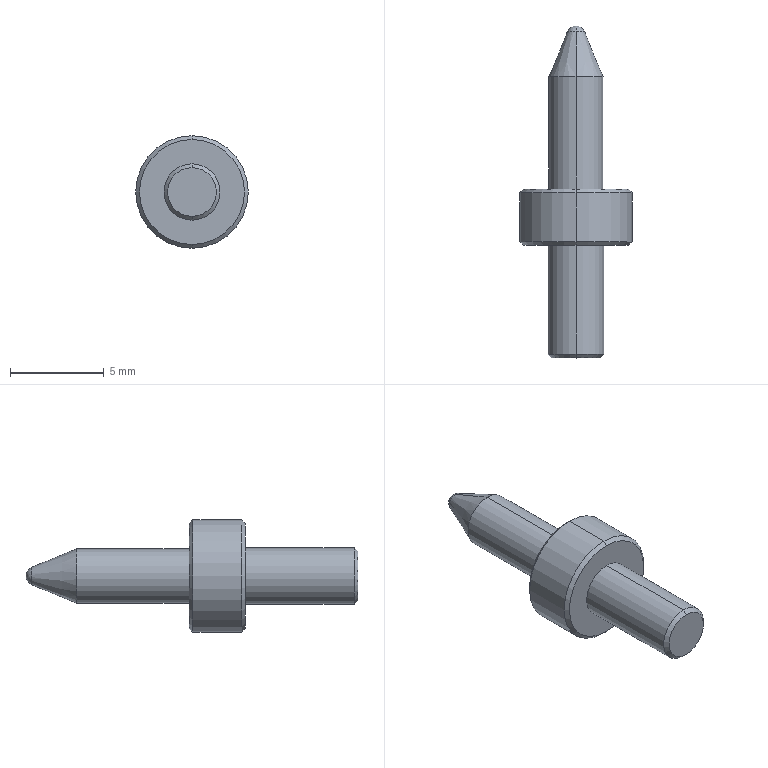Part | STEP file | PN_0028 Pin_Default | 1 solid | 19 faces | box 6 x 17.694 x 6 mm | volume 173.525 mm3 | cone 8 | cylinder 6 | plane 3 | sphere 2 | commonest cylinder face diameters 2.9 x2 3 x2 6 x2
STEP:
#1=CARTESIAN_POINT('',(0.,0.,0.));
#2=DIRECTION('',(0.,0.,1.));
#3=DIRECTION('',(1.,0.,0.));
#4=AXIS2_PLACEMENT_3D('',#1,#2,#3);
#5=CARTESIAN_POINT('',(0.,-6.,-1.3));
#6=VERTEX_POINT('',#5);
#7=CARTESIAN_POINT('',(0.,-6.,1.3));
#8=VERTEX_POINT('',#7);
#9=CARTESIAN_POINT('',(0.,-6.,0.));
#10=DIRECTION('',(0.,-1.,0.));
#11=DIRECTION('',(0.,0.,-1.));
#12=AXIS2_PLACEMENT_3D('',#9,#10,#11);
#13=CIRCLE('',#12,1.3);
#14=CARTESIAN_POINT('',(0.,-6.,0.));
#15=DIRECTION('',(0.,1.,0.));
#16=DIRECTION('',(0.,0.,1.));
#17=AXIS2_PLACEMENT_3D('',#14,#15,#16);
#18=CONICAL_SURFACE('',#17,1.3,0.7854);
#19=CARTESIAN_POINT('',(3.142,0.));
#20=DIRECTION('',(-1.,0.));
#21=VECTOR('',#20,1.);
#22=LINE('',#19,#21);
#23=(GEOMETRIC_REPRESENTATION_CONTEXT(2)PARAMETRIC_REPRESENTATION_CONTEXT()REPRESENTATION_CONTEXT('',''));
#24=DEFINITIONAL_REPRESENTATION('',(#22),#23);
#25=PCURVE('',#18,#24);
#26=CARTESIAN_POINT('',(0.,-6.,0.));
#27=DIRECTION('',(0.,-1.,0.));
#28=DIRECTION('',(0.,0.,-1.));
#29=AXIS2_PLACEMENT_3D('',#26,#27,#28);
#30=PLANE('',#29);
#31=CARTESIAN_POINT('',(0.,0.));
#32=DIRECTION('',(1.,0.));
#33=AXIS2_PLACEMENT_2D('',#31,#32);
#34=CIRCLE('',#33,1.3);
#35=(GEOMETRIC_REPRESENTATION_CONTEXT(2)PARAMETRIC_REPRESENTATION_CONTEXT()REPRESENTATION_CONTEXT('',''));
#36=DEFINITIONAL_REPRESENTATION('',(#34),#35);
#37=PCURVE('',#30,#36);
#38=SURFACE_CURVE('',#13,(#25,#37),.PCURVE_S1.);
#39=EDGE_CURVE('',#6,#8,#38,.T.);
#40=ORIENTED_EDGE('',*,*,#39,.F.);
#41=CARTESIAN_POINT('',(0.,-5.8,-1.5));
#42=VERTEX_POINT('',#41);
#43=CARTESIAN_POINT('',(0.,-6.,-1.3));
#44=DIRECTION('',(0.,0.7071,-0.7071));
#45=VECTOR('',#44,1.);
#46=LINE('',#43,#45);
#47=CARTESIAN_POINT('',(3.142,0.));
#48=DIRECTION('',(0.,1.));
#49=VECTOR('',#48,1.);
#50=LINE('',#47,#49);
#51=(GEOMETRIC_REPRESENTATION_CONTEXT(2)PARAMETRIC_REPRESENTATION_CONTEXT()REPRESENTATION_CONTEXT('',''));
#52=DEFINITIONAL_REPRESENTATION('',(#50),#51);
#53=PCURVE('',#18,#52);
#54=CARTESIAN_POINT('',(0.,-6.,0.));
#55=DIRECTION('',(0.,1.,0.));
#56=DIRECTION('',(0.,0.,1.));
#57=AXIS2_PLACEMENT_3D('',#54,#55,#56);
#58=CONICAL_SURFACE('',#57,1.3,0.7854);
#59=CARTESIAN_POINT('',(3.142,0.));
#60=DIRECTION('',(0.,1.));
#61=VECTOR('',#60,1.);
#62=LINE('',#59,#61);
#63=(GEOMETRIC_REPRESENTATION_CONTEXT(2)PARAMETRIC_REPRESENTATION_CONTEXT()REPRESENTATION_CONTEXT('',''));
#64=DEFINITIONAL_REPRESENTATION('',(#62),#63);
#65=PCURVE('',#58,#64);
#66=SURFACE_CURVE('',#46,(#53,#65),.PCURVE_S1.);
#67=EDGE_CURVE('',#6,#42,#66,.T.);
#68=ORIENTED_EDGE('',*,*,#67,.T.);
#69=CARTESIAN_POINT('',(0.,-5.8,1.5));
#70=VERTEX_POINT('',#69);
#71=CARTESIAN_POINT('',(0.,-5.8,0.));
#72=DIRECTION('',(0.,1.,0.));
#73=DIRECTION('',(0.,0.,-1.));
#74=AXIS2_PLACEMENT_3D('',#71,#72,#73);
#75=CIRCLE('',#74,1.5);
#76=CARTESIAN_POINT('',(-3.142,0.2));
#77=DIRECTION('',(1.,0.));
#78=VECTOR('',#77,1.);
#79=LINE('',#76,#78);
#80=(GEOMETRIC_REPRESENTATION_CONTEXT(2)PARAMETRIC_REPRESENTATION_CONTEXT()REPRESENTATION_CONTEXT('',''));
#81=DEFINITIONAL_REPRESENTATION('',(#79),#80);
#82=PCURVE('',#18,#81);
#83=CARTESIAN_POINT('',(0.,-6.,0.));
#84=DIRECTION('',(0.,1.,0.));
#85=DIRECTION('',(0.,0.,1.));
#86=AXIS2_PLACEMENT_3D('',#83,#84,#85);
#87=CYLINDRICAL_SURFACE('',#86,1.5);
#88=CARTESIAN_POINT('',(-3.142,0.2));
#89=DIRECTION('',(1.,0.));
#90=VECTOR('',#89,1.);
#91=LINE('',#88,#90);
#92=(GEOMETRIC_REPRESENTATION_CONTEXT(2)PARAMETRIC_REPRESENTATION_CONTEXT()REPRESENTATION_CONTEXT('',''));
#93=DEFINITIONAL_REPRESENTATION('',(#91),#92);
#94=PCURVE('',#87,#93);
#95=SURFACE_CURVE('',#75,(#82,#94),.PCURVE_S1.);
#96=EDGE_CURVE('',#70,#42,#95,.T.);
#97=ORIENTED_EDGE('',*,*,#96,.F.);
#98=CARTESIAN_POINT('',(0.,-6.,1.3));
#99=DIRECTION('',(0.,0.7071,0.7071));
#100=VECTOR('',#99,1.);
#101=LINE('',#98,#100);
#102=CARTESIAN_POINT('',(0.,0.));
#103=DIRECTION('',(0.,1.));
#104=VECTOR('',#103,1.);
#105=LINE('',#102,#104);
#106=(GEOMETRIC_REPRESENTATION_CONTEXT(2)PARAMETRIC_REPRESENTATION_CONTEXT()REPRESENTATION_CONTEXT('',''));
#107=DEFINITIONAL_REPRESENTATION('',(#105),#106);
#108=PCURVE('',#18,#107);
#109=CARTESIAN_POINT('',(6.283,0.));
#110=DIRECTION('',(0.,1.));
#111=VECTOR('',#110,1.);
#112=LINE('',#109,#111);
#113=(GEOMETRIC_REPRESENTATION_CONTEXT(2)PARAMETRIC_REPRESENTATION_CONTEXT()REPRESENTATION_CONTEXT('',''));
#114=DEFINITIONAL_REPRESENTATION('',(#112),#113);
#115=PCURVE('',#58,#114);
#116=SURFACE_CURVE('',#101,(#108,#115),.PCURVE_S1.);
#117=EDGE_CURVE('',#8,#70,#116,.T.);
#118=ORIENTED_EDGE('',*,*,#117,.F.);
#119=EDGE_LOOP('',(#40,#68,#97,#118));
#120=FACE_BOUND('',#119,.T.);
#121=ADVANCED_FACE('',(#120),#18,.T.);
#122=CARTESIAN_POINT('',(0.,0.,-2.8));
#123=VERTEX_POINT('',#122);
#124=CARTESIAN_POINT('',(0.,0.,2.8));
#125=VERTEX_POINT('',#124);
#126=CARTESIAN_POINT('',(0.,0.,0.));
#127=DIRECTION('',(0.,-1.,0.));
#128=DIRECTION('',(0.,0.,-1.));
#129=AXIS2_PLACEMENT_3D('',#126,#127,#128);
#130=CIRCLE('',#129,2.8);
#131=CARTESIAN_POINT('',(0.,0.2,0.));
#132=DIRECTION('',(0.,1.,0.));
#133=DIRECTION('',(0.,0.,1.));
#134=AXIS2_PLACEMENT_3D('',#131,#132,#133);
#135=CONICAL_SURFACE('',#134,3.,0.7854);
#136=CARTESIAN_POINT('',(3.142,-0.2));
#137=DIRECTION('',(-1.,0.));
#138=VECTOR('',#137,1.);
#139=LINE('',#136,#138);
#140=(GEOMETRIC_REPRESENTATION_CONTEXT(2)PARAMETRIC_REPRESENTATION_CONTEXT()REPRESENTATION_CONTEXT('',''));
#141=DEFINITIONAL_REPRESENTATION('',(#139),#140);
#142=PCURVE('',#135,#141);
#143=CARTESIAN_POINT('',(0.,0.,3.));
#144=DIRECTION('',(0.,-1.,0.));
#145=DIRECTION('',(0.,0.,-1.));
#146=AXIS2_PLACEMENT_3D('',#143,#144,#145);
#147=PLANE('',#146);
#148=CARTESIAN_POINT('',(3.,0.));
#149=DIRECTION('',(1.,0.));
#150=AXIS2_PLACEMENT_2D('',#148,#149);
#151=CIRCLE('',#150,2.8);
#152=(GEOMETRIC_REPRESENTATION_CONTEXT(2)PARAMETRIC_REPRESENTATION_CONTEXT()REPRESENTATION_CONTEXT('',''));
#153=DEFINITIONAL_REPRESENTATION('',(#151),#152);
#154=PCURVE('',#147,#153);
#155=SURFACE_CURVE('',#130,(#142,#154),.PCURVE_S1.);
#156=EDGE_CURVE('',#123,#125,#155,.T.);
#157=ORIENTED_EDGE('',*,*,#156,.F.);
#158=CARTESIAN_POINT('',(0.,0.2,-3.));
#159=VERTEX_POINT('',#158);
#160=CARTESIAN_POINT('',(0.,0.2,-3.));
#161=DIRECTION('',(0.,0.7071,-0.7071));
#162=VECTOR('',#161,1.);
#163=LINE('',#160,#162);
#164=CARTESIAN_POINT('',(3.142,0.));
#165=DIRECTION('',(0.,1.));
#166=VECTOR('',#165,1.);
#167=LINE('',#164,#166);
#168=(GEOMETRIC_REPRESENTATION_CONTEXT(2)PARAMETRIC_REPRESENTATION_CONTEXT()REPRESENTATION_CONTEXT('',''));
#169=DEFINITIONAL_REPRESENTATION('',(#167),#168);
#170=PCURVE('',#135,#169);
#171=CARTESIAN_POINT('',(0.,0.2,0.));
#172=DIRECTION('',(0.,1.,0.));
#173=DIRECTION('',(0.,0.,1.));
#174=AXIS2_PLACEMENT_3D('',#171,#172,#173);
#175=CONICAL_SURFACE('',#174,3.,0.7854);
#176=CARTESIAN_POINT('',(3.142,0.));
#177=DIRECTION('',(0.,1.));
#178=VECTOR('',#177,1.);
#179=LINE('',#176,#178);
#180=(GEOMETRIC_REPRESENTATION_CONTEXT(2)PARAMETRIC_REPRESENTATION_CONTEXT()REPRESENTATION_CONTEXT('',''));
#181=DEFINITIONAL_REPRESENTATION('',(#179),#180);
#182=PCURVE('',#175,#181);
#183=SURFACE_CURVE('',#163,(#170,#182),.PCURVE_S1.);
#184=EDGE_CURVE('',#123,#159,#183,.T.);
#185=ORIENTED_EDGE('',*,*,#184,.T.);
#186=CARTESIAN_POINT('',(0.,0.2,3.));
#187=VERTEX_POINT('',#186);
#188=CARTESIAN_POINT('',(0.,0.2,0.));
#189=DIRECTION('',(0.,1.,0.));
#190=DIRECTION('',(0.,0.,-1.));
#191=AXIS2_PLACEMENT_3D('',#188,#189,#190);
#192=CIRCLE('',#191,3.);
#193=CARTESIAN_POINT('',(-3.142,0.));
#194=DIRECTION('',(1.,0.));
#195=VECTOR('',#194,1.);
#196=LINE('',#193,#195);
#197=(GEOMETRIC_REPRESENTATION_CONTEXT(2)PARAMETRIC_REPRESENTATION_CONTEXT()REPRESENTATION_CONTEXT('',''));
#198=DEFINITIONAL_REPRESENTATION('',(#196),#197);
#199=PCURVE('',#135,#198);
#200=CARTESIAN_POINT('',(0.,11.694,0.));
#201=DIRECTION('',(0.,1.,0.));
#202=DIRECTION('',(0.,0.,1.));
#203=AXIS2_PLACEMENT_3D('',#200,#201,#202);
#204=CYLINDRICAL_SURFACE('',#203,3.);
#205=CARTESIAN_POINT('',(-3.142,-11.494));
#206=DIRECTION('',(1.,0.));
#207=VECTOR('',#206,1.);
#208=LINE('',#205,#207);
#209=(GEOMETRIC_REPRESENTATION_CONTEXT(2)PARAMETRIC_REPRESENTATION_CONTEXT()REPRESENTATION_CONTEXT('',''));
#210=DEFINITIONAL_REPRESENTATION('',(#208),#209);
#211=PCURVE('',#204,#210);
#212=SURFACE_CURVE('',#192,(#199,#211),.PCURVE_S1.);
#213=EDGE_CURVE('',#187,#159,#212,.T.);
#214=ORIENTED_EDGE('',*,*,#213,.F.);
#215=CARTESIAN_POINT('',(0.,0.2,3.));
#216=DIRECTION('',(0.,0.7071,0.7071));
#217=VECTOR('',#216,1.);
#218=LINE('',#215,#217);
#219=CARTESIAN_POINT('',(0.,0.));
#220=DIRECTION('',(0.,1.));
#221=VECTOR('',#220,1.);
#222=LINE('',#219,#221);
#223=(GEOMETRIC_REPRESENTATION_CONTEXT(2)PARAMETRIC_REPRESENTATION_CONTEXT()REPRESENTATION_CONTEXT('',''));
#224=DEFINITIONAL_REPRESENTATION('',(#222),#223);
#225=PCURVE('',#135,#224);
#226=CARTESIAN_POINT('',(6.283,0.));
#227=DIRECTION('',(0.,1.));
#228=VECTOR('',#227,1.);
#229=LINE('',#226,#228);
#230=(GEOMETRIC_REPRESENTATION_CONTEXT(2)PARAMETRIC_REPRESENTATION_CONTEXT()REPRESENTATION_CONTEXT('',''));
#231=DEFINITIONAL_REPRESENTATION('',(#229),#230);
#232=PCURVE('',#175,#231);
#233=SURFACE_CURVE('',#218,(#225,#232),.PCURVE_S1.);
#234=EDGE_CURVE('',#125,#187,#233,.T.);
#235=ORIENTED_EDGE('',*,*,#234,.F.);
#236=EDGE_LOOP('',(#157,#185,#214,#235));
#237=FACE_BOUND('',#236,.T.);
#238=ADVANCED_FACE('',(#237),#135,.T.);
#239=CARTESIAN_POINT('',(0.,3.,2.8));
#240=VERTEX_POINT('',#239);
#241=CARTESIAN_POINT('',(0.,3.,-2.8));
#242=VERTEX_POINT('',#241);
#243=CARTESIAN_POINT('',(0.,3.,0.));
#244=DIRECTION('',(0.,1.,0.));
#245=DIRECTION('',(0.,0.,1.));
#246=AXIS2_PLACEMENT_3D('',#243,#244,#245);
#247=CIRCLE('',#246,2.8);
#248=CARTESIAN_POINT('',(0.,3.,0.));
#249=DIRECTION('',(0.,-1.,0.));
#250=DIRECTION('',(0.,0.,-1.));
#251=AXIS2_PLACEMENT_3D('',#248,#249,#250);
#252=CONICAL_SURFACE('',#251,2.8,0.7854);
#253=CARTESIAN_POINT('',(3.142,0.));
#254=DIRECTION('',(-1.,0.));
#255=VECTOR('',#254,1.);
#256=LINE('',#253,#255);
#257=(GEOMETRIC_REPRESENTATION_CONTEXT(2)PARAMETRIC_REPRESENTATION_CONTEXT()REPRESENTATION_CONTEXT('',''));
#258=DEFINITIONAL_REPRESENTATION('',(#256),#257);
#259=PCURVE('',#252,#258);
#260=CARTESIAN_POINT('',(0.,3.,1.45));
#261=DIRECTION('',(0.,1.,0.));
#262=DIRECTION('',(0.,0.,1.));
#263=AXIS2_PLACEMENT_3D('',#260,#261,#262);
#264=PLANE('',#263);
#265=CARTESIAN_POINT('',(-1.45,0.));
#266=DIRECTION('',(1.,0.));
#267=AXIS2_PLACEMENT_2D('',#265,#266);
#268=CIRCLE('',#267,2.8);
#269=(GEOMETRIC_REPRESENTATION_CONTEXT(2)PARAMETRIC_REPRESENTATION_CONTEXT()REPRESENTATION_CONTEXT('',''));
#270=DEFINITIONAL_REPRESENTATION('',(#268),#269);
#271=PCURVE('',#264,#270);
#272=SURFACE_CURVE('',#247,(#259,#271),.PCURVE_S1.);
#273=EDGE_CURVE('',#240,#242,#272,.T.);
#274=ORIENTED_EDGE('',*,*,#273,.F.);
#275=CARTESIAN_POINT('',(0.,2.8,3.));
#276=VERTEX_POINT('',#275);
#277=CARTESIAN_POINT('',(0.,3.,2.8));
#278=DIRECTION('',(0.,-0.7071,0.7071));
#279=VECTOR('',#278,1.);
#280=LINE('',#277,#279);
#281=CARTESIAN_POINT('',(3.142,0.));
#282=DIRECTION('',(0.,1.));
#283=VECTOR('',#282,1.);
#284=LINE('',#281,#283);
#285=(GEOMETRIC_REPRESENTATION_CONTEXT(2)PARAMETRIC_REPRESENTATION_CONTEXT()REPRESENTATION_CONTEXT('',''));
#286=DEFINITIONAL_REPRESENTATION('',(#284),#285);
#287=PCURVE('',#252,#286);
#288=CARTESIAN_POINT('',(0.,3.,0.));
#289=DIRECTION('',(0.,-1.,0.));
#290=DIRECTION('',(0.,0.,-1.));
#291=AXIS2_PLACEMENT_3D('',#288,#289,#290);
#292=CONICAL_SURFACE('',#291,2.8,0.7854);
#293=CARTESIAN_POINT('',(3.142,0.));
#294=DIRECTION('',(0.,1.));
#295=VECTOR('',#294,1.);
#296=LINE('',#293,#295);
#297=(GEOMETRIC_REPRESENTATION_CONTEXT(2)PARAMETRIC_REPRESENTATION_CONTEXT()REPRESENTATION_CONTEXT('',''));
#298=DEFINITIONAL_REPRESENTATION('',(#296),#297);
#299=PCURVE('',#292,#298);
#300=SURFACE_CURVE('',#280,(#287,#299),.PCURVE_S1.);
#301=EDGE_CURVE('',#240,#276,#300,.T.);
#302=ORIENTED_EDGE('',*,*,#301,.T.);
#303=CARTESIAN_POINT('',(0.,2.8,-3.));
#304=VERTEX_POINT('',#303);
#305=CARTESIAN_POINT('',(0.,2.8,0.));
#306=DIRECTION('',(0.,-1.,0.));
#307=DIRECTION('',(0.,0.,1.));
#308=AXIS2_PLACEMENT_3D('',#305,#306,#307);
#309=CIRCLE('',#308,3.);
#310=CARTESIAN_POINT('',(-3.142,0.2));
#311=DIRECTION('',(1.,0.));
#312=VECTOR('',#311,1.);
#313=LINE('',#310,#312);
#314=(GEOMETRIC_REPRESENTATION_CONTEXT(2)PARAMETRIC_REPRESENTATION_CONTEXT()REPRESENTATION_CONTEXT('',''));
#315=DEFINITIONAL_REPRESENTATION('',(#313),#314);
#316=PCURVE('',#252,#315);
#317=CARTESIAN_POINT('',(6.283,-8.894));
#318=DIRECTION('',(-1.,0.));
#319=VECTOR('',#318,1.);
#320=LINE('',#317,#319);
#321=(GEOMETRIC_REPRESENTATION_CONTEXT(2)PARAMETRIC_REPRESENTATION_CONTEXT()REPRESENTATION_CONTEXT('',''));
#322=DEFINITIONAL_REPRESENTATION('',(#320),#321);
#323=PCURVE('',#204,#322);
#324=SURFACE_CURVE('',#309,(#316,#323),.PCURVE_S1.);
#325=EDGE_CURVE('',#304,#276,#324,.T.);
#326=ORIENTED_EDGE('',*,*,#325,.F.);
#327=CARTESIAN_POINT('',(0.,3.,-2.8));
#328=DIRECTION('',(0.,-0.7071,-0.7071));
#329=VECTOR('',#328,1.);
#330=LINE('',#327,#329);
#331=CARTESIAN_POINT('',(0.,0.));
#332=DIRECTION('',(0.,1.));
#333=VECTOR('',#332,1.);
#334=LINE('',#331,#333);
#335=(GEOMETRIC_REPRESENTATION_CONTEXT(2)PARAMETRIC_REPRESENTATION_CONTEXT()REPRESENTATION_CONTEXT('',''));
#336=DEFINITIONAL_REPRESENTATION('',(#334),#335);
#337=PCURVE('',#252,#336);
#338=CARTESIAN_POINT('',(6.283,0.));
#339=DIRECTION('',(0.,1.));
#340=VECTOR('',#339,1.);
#341=LINE('',#338,#340);
#342=(GEOMETRIC_REPRESENTATION_CONTEXT(2)PARAMETRIC_REPRESENTATION_CONTEXT()REPRESENTATION_CONTEXT('',''));
#343=DEFINITIONAL_REPRESENTATION('',(#341),#342);
#344=PCURVE('',#292,#343);
#345=SURFACE_CURVE('',#330,(#337,#344),.PCURVE_S1.);
#346=EDGE_CURVE('',#242,#304,#345,.T.);
#347=ORIENTED_EDGE('',*,*,#346,.F.);
#348=EDGE_LOOP('',(#274,#302,#326,#347));
#349=FACE_BOUND('',#348,.T.);
#350=ADVANCED_FACE('',(#349),#252,.T.);
#351=ORIENTED_EDGE('',*,*,#96,.T.);
#352=CARTESIAN_POINT('',(0.,0.,-1.5));
#353=VERTEX_POINT('',#352);
#354=CARTESIAN_POINT('',(0.,-6.,-1.5));
#355=DIRECTION('',(0.,1.,0.));
#356=VECTOR('',#355,1.);
#357=LINE('',#354,#356);
#358=CARTESIAN_POINT('',(3.142,0.));
#359=DIRECTION('',(0.,1.));
#360=VECTOR('',#359,1.);
#361=LINE('',#358,#360);
#362=(GEOMETRIC_REPRESENTATION_CONTEXT(2)PARAMETRIC_REPRESENTATION_CONTEXT()REPRESENTATION_CONTEXT('',''));
#363=DEFINITIONAL_REPRESENTATION('',(#361),#362);
#364=PCURVE('',#87,#363);
#365=CARTESIAN_POINT('',(0.,-6.,0.));
#366=DIRECTION('',(0.,1.,0.));
#367=DIRECTION('',(0.,0.,1.));
#368=AXIS2_PLACEMENT_3D('',#365,#366,#367);
#369=CYLINDRICAL_SURFACE('',#368,1.5);
#370=CARTESIAN_POINT('',(3.142,0.));
#371=DIRECTION('',(0.,1.));
#372=VECTOR('',#371,1.);
#373=LINE('',#370,#372);
#374=(GEOMETRIC_REPRESENTATION_CONTEXT(2)PARAMETRIC_REPRESENTATION_CONTEXT()REPRESENTATION_CONTEXT('',''));
#375=DEFINITIONAL_REPRESENTATION('',(#373),#374);
#376=PCURVE('',#369,#375);
#377=SURFACE_CURVE('',#357,(#364,#376),.PCURVE_S1.);
#378=EDGE_CURVE('',#42,#353,#377,.T.);
#379=ORIENTED_EDGE('',*,*,#378,.T.);
#380=CARTESIAN_POINT('',(0.,0.,1.5));
#381=VERTEX_POINT('',#380);
#382=CARTESIAN_POINT('',(0.,0.,0.));
#383=DIRECTION('',(0.,-1.,0.));
#384=DIRECTION('',(0.,0.,-1.));
#385=AXIS2_PLACEMENT_3D('',#382,#383,#384);
#386=CIRCLE('',#385,1.5);
#387=CARTESIAN_POINT('',(3.142,6.));
#388=DIRECTION('',(-1.,0.));
#389=VECTOR('',#388,1.);
#390=LINE('',#387,#389);
#391=(GEOMETRIC_REPRESENTATION_CONTEXT(2)PARAMETRIC_REPRESENTATION_CONTEXT()REPRESENTATION_CONTEXT('',''));
#392=DEFINITIONAL_REPRESENTATION('',(#390),#391);
#393=PCURVE('',#87,#392);
#394=CARTESIAN_POINT('',(3.,0.));
#395=DIRECTION('',(1.,0.));
#396=AXIS2_PLACEMENT_2D('',#394,#395);
#397=CIRCLE('',#396,1.5);
#398=(GEOMETRIC_REPRESENTATION_CONTEXT(2)PARAMETRIC_REPRESENTATION_CONTEXT()REPRESENTATION_CONTEXT('',''));
#399=DEFINITIONAL_REPRESENTATION('',(#397),#398);
#400=PCURVE('',#147,#399);
#401=SURFACE_CURVE('',#386,(#393,#400),.PCURVE_S1.);
#402=EDGE_CURVE('',#353,#381,#401,.T.);
#403=ORIENTED_EDGE('',*,*,#402,.T.);
#404=CARTESIAN_POINT('',(0.,-6.,1.5));
#405=DIRECTION('',(0.,1.,0.));
#406=VECTOR('',#405,1.);
#407=LINE('',#404,#406);
#408=CARTESIAN_POINT('',(0.,0.));
#409=DIRECTION('',(0.,1.));
#410=VECTOR('',#409,1.);
#411=LINE('',#408,#410);
#412=(GEOMETRIC_REPRESENTATION_CONTEXT(2)PARAMETRIC_REPRESENTATION_CONTEXT()REPRESENTATION_CONTEXT('',''));
#413=DEFINITIONAL_REPRESENTATION('',(#411),#412);
#414=PCURVE('',#87,#413);
#415=CARTESIAN_POINT('',(6.283,0.));
#416=DIRECTION('',(0.,1.));
#417=VECTOR('',#416,1.);
#418=LINE('',#415,#417);
#419=(GEOMETRIC_REPRESENTATION_CONTEXT(2)PARAMETRIC_REPRESENTATION_CONTEXT()REPRESENTATION_CONTEXT('',''));
#420=DEFINITIONAL_REPRESENTATION('',(#418),#419);
#421=PCURVE('',#369,#420);
#422=SURFACE_CURVE('',#407,(#414,#421),.PCURVE_S1.);
#423=EDGE_CURVE('',#70,#381,#422,.T.);
#424=ORIENTED_EDGE('',*,*,#423,.F.);
#425=EDGE_LOOP('',(#351,#379,#403,#424));
#426=FACE_BOUND('',#425,.T.);
#427=ADVANCED_FACE('',(#426),#87,.T.);
#428=CARTESIAN_POINT('',(0.,3.,1.45));
#429=VERTEX_POINT('',#428);
#430=CARTESIAN_POINT('',(0.,3.,-1.45));
#431=VERTEX_POINT('',#430);
#432=CARTESIAN_POINT('',(0.,3.,0.));
#433=DIRECTION('',(0.,1.,0.));
#434=DIRECTION('',(0.,0.,1.));
#435=AXIS2_PLACEMENT_3D('',#432,#433,#434);
#436=CIRCLE('',#435,1.45);
#437=CARTESIAN_POINT('',(0.,11.694,0.));
#438=DIRECTION('',(0.,1.,0.));
#439=DIRECTION('',(0.,0.,1.));
#440=AXIS2_PLACEMENT_3D('',#437,#438,#439);
#441=CYLINDRICAL_SURFACE('',#440,1.45);
#442=CARTESIAN_POINT('',(0.,-8.694));
#443=DIRECTION('',(1.,0.));
#444=VECTOR('',#443,1.);
#445=LINE('',#442,#444);
#446=(GEOMETRIC_REPRESENTATION_CONTEXT(2)PARAMETRIC_REPRESENTATION_CONTEXT()REPRESENTATION_CONTEXT('',''));
#447=DEFINITIONAL_REPRESENTATION('',(#445),#446);
#448=PCURVE('',#441,#447);
#449=CARTESIAN_POINT('',(-1.45,0.));
#450=DIRECTION('',(1.,0.));
#451=AXIS2_PLACEMENT_2D('',#449,#450);
#452=CIRCLE('',#451,1.45);
#453=(GEOMETRIC_REPRESENTATION_CONTEXT(2)PARAMETRIC_REPRESENTATION_CONTEXT()REPRESENTATION_CONTEXT('',''));
#454=DEFINITIONAL_REPRESENTATION('',(#452),#453);
#455=PCURVE('',#264,#454);
#456=SURFACE_CURVE('',#436,(#448,#455),.PCURVE_S1.);
#457=EDGE_CURVE('',#429,#431,#456,.T.);
#458=ORIENTED_EDGE('',*,*,#457,.T.);
#459=CARTESIAN_POINT('',(0.,9.,-1.45));
#460=VERTEX_POINT('',#459);
#461=CARTESIAN_POINT('',(0.,11.694,-1.45));
#462=DIRECTION('',(0.,1.,0.));
#463=VECTOR('',#462,1.);
#464=LINE('',#461,#463);
#465=CARTESIAN_POINT('',(3.142,0.));
#466=DIRECTION('',(0.,1.));
#467=VECTOR('',#466,1.);
#468=LINE('',#465,#467);
#469=(GEOMETRIC_REPRESENTATION_CONTEXT(2)PARAMETRIC_REPRESENTATION_CONTEXT()REPRESENTATION_CONTEXT('',''));
#470=DEFINITIONAL_REPRESENTATION('',(#468),#469);
#471=PCURVE('',#441,#470);
#472=CARTESIAN_POINT('',(0.,11.694,0.));
#473=DIRECTION('',(0.,1.,0.));
#474=DIRECTION('',(0.,0.,1.));
#475=AXIS2_PLACEMENT_3D('',#472,#473,#474);
#476=CYLINDRICAL_SURFACE('',#475,1.45);
#477=CARTESIAN_POINT('',(3.142,0.));
#478=DIRECTION('',(0.,1.));
#479=VECTOR('',#478,1.);
#480=LINE('',#477,#479);
#481=(GEOMETRIC_REPRESENTATION_CONTEXT(2)PARAMETRIC_REPRESENTATION_CONTEXT()REPRESENTATION_CONTEXT('',''));
#482=DEFINITIONAL_REPRESENTATION('',(#480),#481);
#483=PCURVE('',#476,#482);
#484=SURFACE_CURVE('',#464,(#471,#483),.PCURVE_S1.);
#485=EDGE_CURVE('',#431,#460,#484,.T.);
#486=ORIENTED_EDGE('',*,*,#485,.T.);
#487=CARTESIAN_POINT('',(0.,9.,1.45));
#488=VERTEX_POINT('',#487);
#489=CARTESIAN_POINT('',(0.,9.,0.));
#490=DIRECTION('',(0.,1.,0.));
#491=DIRECTION('',(0.,0.,1.));
#492=AXIS2_PLACEMENT_3D('',#489,#490,#491);
#493=CIRCLE('',#492,1.45);
#494=CARTESIAN_POINT('',(0.,-2.694));
#495=DIRECTION('',(1.,0.));
#496=VECTOR('',#495,1.);
#497=LINE('',#494,#496);
#498=(GEOMETRIC_REPRESENTATION_CONTEXT(2)PARAMETRIC_REPRESENTATION_CONTEXT()REPRESENTATION_CONTEXT('',''));
#499=DEFINITIONAL_REPRESENTATION('',(#497),#498);
#500=PCURVE('',#441,#499);
#501=CARTESIAN_POINT('',(0.,11.385,0.));
#502=DIRECTION('',(0.,-1.,0.));
#503=DIRECTION('',(0.,0.,-1.));
#504=AXIS2_PLACEMENT_3D('',#501,#502,#503);
#505=CONICAL_SURFACE('',#504,0.4619,0.3927);
#506=CARTESIAN_POINT('',(3.142,2.385));
#507=DIRECTION('',(-1.,0.));
#508=VECTOR('',#507,1.);
#509=LINE('',#506,#508);
#510=(GEOMETRIC_REPRESENTATION_CONTEXT(2)PARAMETRIC_REPRESENTATION_CONTEXT()REPRESENTATION_CONTEXT('',''));
#511=DEFINITIONAL_REPRESENTATION('',(#509),#510);
#512=PCURVE('',#505,#511);
#513=SURFACE_CURVE('',#493,(#500,#512),.PCURVE_S1.);
#514=EDGE_CURVE('',#488,#460,#513,.T.);
#515=ORIENTED_EDGE('',*,*,#514,.F.);
#516=CARTESIAN_POINT('',(0.,11.694,1.45));
#517=DIRECTION('',(0.,1.,0.));
#518=VECTOR('',#517,1.);
#519=LINE('',#516,#518);
#520=CARTESIAN_POINT('',(0.,0.));
#521=DIRECTION('',(0.,1.));
#522=VECTOR('',#521,1.);
#523=LINE('',#520,#522);
#524=(GEOMETRIC_REPRESENTATION_CONTEXT(2)PARAMETRIC_REPRESENTATION_CONTEXT()REPRESENTATION_CONTEXT('',''));
#525=DEFINITIONAL_REPRESENTATION('',(#523),#524);
#526=PCURVE('',#441,#525);
#527=CARTESIAN_POINT('',(6.283,0.));
#528=DIRECTION('',(0.,1.));
#529=VECTOR('',#528,1.);
#530=LINE('',#527,#529);
#531=(GEOMETRIC_REPRESENTATION_CONTEXT(2)PARAMETRIC_REPRESENTATION_CONTEXT()REPRESENTATION_CONTEXT('',''));
#532=DEFINITIONAL_REPRESENTATION('',(#530),#531);
#533=PCURVE('',#476,#532);
#534=SURFACE_CURVE('',#519,(#526,#533),.PCURVE_S1.);
#535=EDGE_CURVE('',#429,#488,#534,.T.);
#536=ORIENTED_EDGE('',*,*,#535,.F.);
#537=EDGE_LOOP('',(#458,#486,#515,#536));
#538=FACE_BOUND('',#537,.T.);
#539=ADVANCED_FACE('',(#538),#441,.T.);
#540=CARTESIAN_POINT('',(0.,11.385,0.4619));
#541=VERTEX_POINT('',#540);
#542=CARTESIAN_POINT('',(0.,11.385,-0.4619));
#543=VERTEX_POINT('',#542);
#544=CARTESIAN_POINT('',(0.,11.385,0.));
#545=DIRECTION('',(0.,1.,0.));
#546=DIRECTION('',(0.,0.,1.));
#547=AXIS2_PLACEMENT_3D('',#544,#545,#546);
#548=CIRCLE('',#547,0.4619);
#549=CARTESIAN_POINT('',(3.142,0.));
#550=DIRECTION('',(-1.,0.));
#551=VECTOR('',#550,1.);
#552=LINE('',#549,#551);
#553=(GEOMETRIC_REPRESENTATION_CONTEXT(2)PARAMETRIC_REPRESENTATION_CONTEXT()REPRESENTATION_CONTEXT('',''));
#554=DEFINITIONAL_REPRESENTATION('',(#552),#553);
#555=PCURVE('',#505,#554);
#556=CARTESIAN_POINT('',(0.,11.194,0.));
#557=DIRECTION('',(1.,0.,0.));
#558=DIRECTION('',(0.,0.,1.));
#559=AXIS2_PLACEMENT_3D('',#556,#557,#558);
#560=SPHERICAL_SURFACE('',#559,0.5);
#561=CARTESIAN_POINT('',(5.89,0.));
#562=CARTESIAN_POINT('',(5.89,0.04397));
#563=CARTESIAN_POINT('',(5.888,0.1319));
#564=CARTESIAN_POINT('',(5.877,0.2635));
#565=CARTESIAN_POINT('',(5.858,0.3941));
#566=CARTESIAN_POINT('',(5.828,0.5234));
#567=CARTESIAN_POINT('',(5.785,0.6504));
#568=CARTESIAN_POINT('',(5.724,0.7738));
#569=CARTESIAN_POINT('',(5.636,0.8917));
#570=CARTESIAN_POINT('',(5.509,1.001));
#571=CARTESIAN_POINT('',(5.323,1.094));
#572=CARTESIAN_POINT('',(5.056,1.161));
#573=CARTESIAN_POINT('',(4.712,1.187));
#574=CARTESIAN_POINT('',(4.369,1.161));
#575=CARTESIAN_POINT('',(4.102,1.094));
#576=CARTESIAN_POINT('',(3.916,1.001));
#577=CARTESIAN_POINT('',(3.789,0.8917));
#578=CARTESIAN_POINT('',(3.701,0.7738));
#579=CARTESIAN_POINT('',(3.64,0.6504));
#580=CARTESIAN_POINT('',(3.597,0.5234));
#581=CARTESIAN_POINT('',(3.567,0.3941));
#582=CARTESIAN_POINT('',(3.548,0.2635));
#583=CARTESIAN_POINT('',(3.537,0.1319));
#584=CARTESIAN_POINT('',(3.534,0.04397));
#585=CARTESIAN_POINT('',(3.534,0.));
#586=B_SPLINE_CURVE_WITH_KNOTS('',3,(#561,#562,#563,#564,#565,#566,#567,#568,#569,#570,#571,#572,#573,#574,#575,#576,#577,#578,#579,#580,#581,#582,#583,#584,#585),.UNSPECIFIED.,.F.,.F.,(4,1,1,1,1,1,1,1,1,1,1,1,1,1,1,1,1,1,1,1,1,1,4),(0.,0.1428,0.2856,0.4284,0.5712,0.714,0.8568,0.9996,1.142,1.285,1.428,1.571,1.714,1.856,1.999,2.142,2.285,2.428,2.57,2.713,2.856,2.999,3.142),.QUASI_UNIFORM_KNOTS.);
#587=(GEOMETRIC_REPRESENTATION_CONTEXT(2)PARAMETRIC_REPRESENTATION_CONTEXT()REPRESENTATION_CONTEXT('',''));
#588=DEFINITIONAL_REPRESENTATION('',(#586),#587);
#589=PCURVE('',#560,#588);
#590=SURFACE_CURVE('',#548,(#555,#589),.PCURVE_S1.);
#591=EDGE_CURVE('',#541,#543,#590,.T.);
#592=ORIENTED_EDGE('',*,*,#591,.F.);
#593=CARTESIAN_POINT('',(0.,11.385,0.4619));
#594=DIRECTION('',(0.,-0.9239,0.3827));
#595=VECTOR('',#594,1.);
#596=LINE('',#593,#595);
#597=CARTESIAN_POINT('',(3.142,0.));
#598=DIRECTION('',(0.,1.));
#599=VECTOR('',#598,1.);
#600=LINE('',#597,#599);
#601=(GEOMETRIC_REPRESENTATION_CONTEXT(2)PARAMETRIC_REPRESENTATION_CONTEXT()REPRESENTATION_CONTEXT('',''));
#602=DEFINITIONAL_REPRESENTATION('',(#600),#601);
#603=PCURVE('',#505,#602);
#604=CARTESIAN_POINT('',(0.,11.385,0.));
#605=DIRECTION('',(0.,-1.,0.));
#606=DIRECTION('',(0.,0.,-1.));
#607=AXIS2_PLACEMENT_3D('',#604,#605,#606);
#608=CONICAL_SURFACE('',#607,0.4619,0.3927);
#609=CARTESIAN_POINT('',(3.142,0.));
#610=DIRECTION('',(0.,1.));
#611=VECTOR('',#610,1.);
#612=LINE('',#609,#611);
#613=(GEOMETRIC_REPRESENTATION_CONTEXT(2)PARAMETRIC_REPRESENTATION_CONTEXT()REPRESENTATION_CONTEXT('',''));
#614=DEFINITIONAL_REPRESENTATION('',(#612),#613);
#615=PCURVE('',#608,#614);
#616=SURFACE_CURVE('',#596,(#603,#615),.PCURVE_S1.);
#617=EDGE_CURVE('',#541,#488,#616,.T.);
#618=ORIENTED_EDGE('',*,*,#617,.T.);
#619=ORIENTED_EDGE('',*,*,#514,.T.);
#620=CARTESIAN_POINT('',(0.,11.385,-0.4619));
#621=DIRECTION('',(0.,-0.9239,-0.3827));
#622=VECTOR('',#621,1.);
#623=LINE('',#620,#622);
#624=CARTESIAN_POINT('',(0.,0.));
#625=DIRECTION('',(0.,1.));
#626=VECTOR('',#625,1.);
#627=LINE('',#624,#626);
#628=(GEOMETRIC_REPRESENTATION_CONTEXT(2)PARAMETRIC_REPRESENTATION_CONTEXT()REPRESENTATION_CONTEXT('',''));
#629=DEFINITIONAL_REPRESENTATION('',(#627),#628);
#630=PCURVE('',#505,#629);
#631=CARTESIAN_POINT('',(6.283,0.));
#632=DIRECTION('',(0.,1.));
#633=VECTOR('',#632,1.);
#634=LINE('',#631,#633);
#635=(GEOMETRIC_REPRESENTATION_CONTEXT(2)PARAMETRIC_REPRESENTATION_CONTEXT()REPRESENTATION_CONTEXT('',''));
#636=DEFINITIONAL_REPRESENTATION('',(#634),#635);
#637=PCURVE('',#608,#636);
#638=SURFACE_CURVE('',#623,(#630,#637),.PCURVE_S1.);
#639=EDGE_CURVE('',#543,#460,#638,.T.);
#640=ORIENTED_EDGE('',*,*,#639,.F.);
#641=EDGE_LOOP('',(#592,#618,#619,#640));
#642=FACE_BOUND('',#641,.T.);
#643=ADVANCED_FACE('',(#642),#505,.T.);
#644=ORIENTED_EDGE('',*,*,#591,.T.);
#645=CARTESIAN_POINT('',(0.,11.694,0.));
#646=VERTEX_POINT('',#645);
#647=CARTESIAN_POINT('',(0.,11.194,0.));
#648=DIRECTION('',(1.,0.,0.));
#649=DIRECTION('',(0.,0.,-1.));
#650=AXIS2_PLACEMENT_3D('',#647,#648,#649);
#651=CIRCLE('',#650,0.5);
#652=CARTESIAN_POINT('',(3.142,0.));
#653=DIRECTION('',(1.,0.));
#654=VECTOR('',#653,1.);
#655=LINE('',#652,#654);
#656=(GEOMETRIC_REPRESENTATION_CONTEXT(2)PARAMETRIC_REPRESENTATION_CONTEXT()REPRESENTATION_CONTEXT('',''));
#657=DEFINITIONAL_REPRESENTATION('',(#655),#656);
#658=PCURVE('',#560,#657);
#659=CARTESIAN_POINT('',(0.,11.194,0.));
#660=DIRECTION('',(1.,0.,0.));
#661=DIRECTION('',(0.,0.,1.));
#662=AXIS2_PLACEMENT_3D('',#659,#660,#661);
#663=SPHERICAL_SURFACE('',#662,0.5);
#664=CARTESIAN_POINT('',(3.142,0.));
#665=DIRECTION('',(1.,0.));
#666=VECTOR('',#665,1.);
#667=LINE('',#664,#666);
#668=(GEOMETRIC_REPRESENTATION_CONTEXT(2)PARAMETRIC_REPRESENTATION_CONTEXT()REPRESENTATION_CONTEXT('',''));
#669=DEFINITIONAL_REPRESENTATION('',(#667),#668);
#670=PCURVE('',#663,#669);
#671=SURFACE_CURVE('',#651,(#658,#670),.PCURVE_S1.);
#672=EDGE_CURVE('',#543,#646,#671,.T.);
#673=ORIENTED_EDGE('',*,*,#672,.T.);
#674=CARTESIAN_POINT('',(0.,11.194,0.));
#675=DIRECTION('',(-1.,0.,0.));
#676=DIRECTION('',(0.,0.,1.));
#677=AXIS2_PLACEMENT_3D('',#674,#675,#676);
#678=CIRCLE('',#677,0.5);
#679=CARTESIAN_POINT('',(6.283,0.));
#680=DIRECTION('',(-1.,0.));
#681=VECTOR('',#680,1.);
#682=LINE('',#679,#681);
#683=(GEOMETRIC_REPRESENTATION_CONTEXT(2)PARAMETRIC_REPRESENTATION_CONTEXT()REPRESENTATION_CONTEXT('',''));
#684=DEFINITIONAL_REPRESENTATION('',(#682),#683);
#685=PCURVE('',#560,#684);
#686=CARTESIAN_POINT('',(6.283,0.));
#687=DIRECTION('',(-1.,0.));
#688=VECTOR('',#687,1.);
#689=LINE('',#686,#688);
#690=(GEOMETRIC_REPRESENTATION_CONTEXT(2)PARAMETRIC_REPRESENTATION_CONTEXT()REPRESENTATION_CONTEXT('',''));
#691=DEFINITIONAL_REPRESENTATION('',(#689),#690);
#692=PCURVE('',#663,#691);
#693=SURFACE_CURVE('',#678,(#685,#692),.PCURVE_S1.);
#694=EDGE_CURVE('',#541,#646,#693,.T.);
#695=ORIENTED_EDGE('',*,*,#694,.F.);
#696=EDGE_LOOP('',(#644,#673,#695));
#697=FACE_BOUND('',#696,.T.);
#698=ADVANCED_FACE('',(#697),#560,.T.);
#699=ORIENTED_EDGE('',*,*,#213,.T.);
#700=CARTESIAN_POINT('',(0.,11.694,-3.));
#701=DIRECTION('',(0.,1.,0.));
#702=VECTOR('',#701,1.);
#703=LINE('',#700,#702);
#704=CARTESIAN_POINT('',(3.142,0.));
#705=DIRECTION('',(0.,1.));
#706=VECTOR('',#705,1.);
#707=LINE('',#704,#706);
#708=(GEOMETRIC_REPRESENTATION_CONTEXT(2)PARAMETRIC_REPRESENTATION_CONTEXT()REPRESENTATION_CONTEXT('',''));
#709=DEFINITIONAL_REPRESENTATION('',(#707),#708);
#710=PCURVE('',#204,#709);
#711=CARTESIAN_POINT('',(0.,11.694,0.));
#712=DIRECTION('',(0.,1.,0.));
#713=DIRECTION('',(0.,0.,1.));
#714=AXIS2_PLACEMENT_3D('',#711,#712,#713);
#715=CYLINDRICAL_SURFACE('',#714,3.);
#716=CARTESIAN_POINT('',(3.142,0.));
#717=DIRECTION('',(0.,1.));
#718=VECTOR('',#717,1.);
#719=LINE('',#716,#718);
#720=(GEOMETRIC_REPRESENTATION_CONTEXT(2)PARAMETRIC_REPRESENTATION_CONTEXT()REPRESENTATION_CONTEXT('',''));
#721=DEFINITIONAL_REPRESENTATION('',(#719),#720);
#722=PCURVE('',#715,#721);
#723=SURFACE_CURVE('',#703,(#710,#722),.PCURVE_S1.);
#724=EDGE_CURVE('',#159,#304,#723,.T.);
#725=ORIENTED_EDGE('',*,*,#724,.T.);
#726=ORIENTED_EDGE('',*,*,#325,.T.);
#727=CARTESIAN_POINT('',(0.,11.694,3.));
#728=DIRECTION('',(0.,1.,0.));
#729=VECTOR('',#728,1.);
#730=LINE('',#727,#729);
#731=CARTESIAN_POINT('',(0.,0.));
#732=DIRECTION('',(0.,1.));
#733=VECTOR('',#732,1.);
#734=LINE('',#731,#733);
#735=(GEOMETRIC_REPRESENTATION_CONTEXT(2)PARAMETRIC_REPRESENTATION_CONTEXT()REPRESENTATION_CONTEXT('',''));
#736=DEFINITIONAL_REPRESENTATION('',(#734),#735);
#737=PCURVE('',#204,#736);
#738=CARTESIAN_POINT('',(6.283,0.));
#739=DIRECTION('',(0.,1.));
#740=VECTOR('',#739,1.);
#741=LINE('',#738,#740);
#742=(GEOMETRIC_REPRESENTATION_CONTEXT(2)PARAMETRIC_REPRESENTATION_CONTEXT()REPRESENTATION_CONTEXT('',''));
#743=DEFINITIONAL_REPRESENTATION('',(#741),#742);
#744=PCURVE('',#715,#743);
#745=SURFACE_CURVE('',#730,(#737,#744),.PCURVE_S1.);
#746=EDGE_CURVE('',#187,#276,#745,.T.);
#747=ORIENTED_EDGE('',*,*,#746,.F.);
#748=EDGE_LOOP('',(#699,#725,#726,#747));
#749=FACE_BOUND('',#748,.T.);
#750=ADVANCED_FACE('',(#749),#204,.T.);
#751=CARTESIAN_POINT('',(0.,0.,0.));
#752=DIRECTION('',(0.,-1.,0.));
#753=DIRECTION('',(0.,0.,-1.));
#754=AXIS2_PLACEMENT_3D('',#751,#752,#753);
#755=CIRCLE('',#754,2.8);
#756=CARTESIAN_POINT('',(3.,0.));
#757=DIRECTION('',(1.,0.));
#758=AXIS2_PLACEMENT_2D('',#756,#757);
#759=CIRCLE('',#758,2.8);
#760=(GEOMETRIC_REPRESENTATION_CONTEXT(2)PARAMETRIC_REPRESENTATION_CONTEXT()REPRESENTATION_CONTEXT('',''));
#761=DEFINITIONAL_REPRESENTATION('',(#759),#760);
#762=PCURVE('',#147,#761);
#763=CARTESIAN_POINT('',(9.425,-0.2));
#764=DIRECTION('',(-1.,0.));
#765=VECTOR('',#764,1.);
#766=LINE('',#763,#765);
#767=(GEOMETRIC_REPRESENTATION_CONTEXT(2)PARAMETRIC_REPRESENTATION_CONTEXT()REPRESENTATION_CONTEXT('',''));
#768=DEFINITIONAL_REPRESENTATION('',(#766),#767);
#769=PCURVE('',#175,#768);
#770=SURFACE_CURVE('',#755,(#762,#769),.PCURVE_S1.);
#771=EDGE_CURVE('',#125,#123,#770,.T.);
#772=ORIENTED_EDGE('',*,*,#771,.T.);
#773=ORIENTED_EDGE('',*,*,#156,.T.);
#774=EDGE_LOOP('',(#772,#773));
#775=FACE_BOUND('',#774,.T.);
#776=CARTESIAN_POINT('',(0.,0.,0.));
#777=DIRECTION('',(0.,-1.,0.));
#778=DIRECTION('',(0.,0.,-1.));
#779=AXIS2_PLACEMENT_3D('',#776,#777,#778);
#780=CIRCLE('',#779,1.5);
#781=CARTESIAN_POINT('',(3.,0.));
#782=DIRECTION('',(1.,0.));
#783=AXIS2_PLACEMENT_2D('',#781,#782);
#784=CIRCLE('',#783,1.5);
#785=(GEOMETRIC_REPRESENTATION_CONTEXT(2)PARAMETRIC_REPRESENTATION_CONTEXT()REPRESENTATION_CONTEXT('',''));
#786=DEFINITIONAL_REPRESENTATION('',(#784),#785);
#787=PCURVE('',#147,#786);
#788=CARTESIAN_POINT('',(9.425,6.));
#789=DIRECTION('',(-1.,0.));
#790=VECTOR('',#789,1.);
#791=LINE('',#788,#790);
#792=(GEOMETRIC_REPRESENTATION_CONTEXT(2)PARAMETRIC_REPRESENTATION_CONTEXT()REPRESENTATION_CONTEXT('',''));
#793=DEFINITIONAL_REPRESENTATION('',(#791),#792);
#794=PCURVE('',#369,#793);
#795=SURFACE_CURVE('',#780,(#787,#794),.PCURVE_S1.);
#796=EDGE_CURVE('',#381,#353,#795,.T.);
#797=ORIENTED_EDGE('',*,*,#796,.F.);
#798=ORIENTED_EDGE('',*,*,#402,.F.);
#799=EDGE_LOOP('',(#797,#798));
#800=FACE_BOUND('',#799,.T.);
#801=ADVANCED_FACE('',(#775,#800),#147,.T.);
#802=CARTESIAN_POINT('',(0.,3.,0.));
#803=DIRECTION('',(0.,1.,0.));
#804=DIRECTION('',(0.,0.,1.));
#805=AXIS2_PLACEMENT_3D('',#802,#803,#804);
#806=CIRCLE('',#805,2.8);
#807=CARTESIAN_POINT('',(-1.45,0.));
#808=DIRECTION('',(1.,0.));
#809=AXIS2_PLACEMENT_2D('',#807,#808);
#810=CIRCLE('',#809,2.8);
#811=(GEOMETRIC_REPRESENTATION_CONTEXT(2)PARAMETRIC_REPRESENTATION_CONTEXT()REPRESENTATION_CONTEXT('',''));
#812=DEFINITIONAL_REPRESENTATION('',(#810),#811);
#813=PCURVE('',#264,#812);
#814=CARTESIAN_POINT('',(9.425,0.));
#815=DIRECTION('',(-1.,0.));
#816=VECTOR('',#815,1.);
#817=LINE('',#814,#816);
#818=(GEOMETRIC_REPRESENTATION_CONTEXT(2)PARAMETRIC_REPRESENTATION_CONTEXT()REPRESENTATION_CONTEXT('',''));
#819=DEFINITIONAL_REPRESENTATION('',(#817),#818);
#820=PCURVE('',#292,#819);
#821=SURFACE_CURVE('',#806,(#813,#820),.PCURVE_S1.);
#822=EDGE_CURVE('',#242,#240,#821,.T.);
#823=ORIENTED_EDGE('',*,*,#822,.T.);
#824=ORIENTED_EDGE('',*,*,#273,.T.);
#825=EDGE_LOOP('',(#823,#824));
#826=FACE_BOUND('',#825,.T.);
#827=ORIENTED_EDGE('',*,*,#457,.F.);
#828=CARTESIAN_POINT('',(0.,3.,0.));
#829=DIRECTION('',(0.,1.,0.));
#830=DIRECTION('',(0.,0.,1.));
#831=AXIS2_PLACEMENT_3D('',#828,#829,#830);
#832=CIRCLE('',#831,1.45);
#833=CARTESIAN_POINT('',(-1.45,0.));
#834=DIRECTION('',(1.,0.));
#835=AXIS2_PLACEMENT_2D('',#833,#834);
#836=CIRCLE('',#835,1.45);
#837=(GEOMETRIC_REPRESENTATION_CONTEXT(2)PARAMETRIC_REPRESENTATION_CONTEXT()REPRESENTATION_CONTEXT('',''));
#838=DEFINITIONAL_REPRESENTATION('',(#836),#837);
#839=PCURVE('',#264,#838);
#840=CARTESIAN_POINT('',(0.,-8.694));
#841=DIRECTION('',(1.,0.));
#842=VECTOR('',#841,1.);
#843=LINE('',#840,#842);
#844=(GEOMETRIC_REPRESENTATION_CONTEXT(2)PARAMETRIC_REPRESENTATION_CONTEXT()REPRESENTATION_CONTEXT('',''));
#845=DEFINITIONAL_REPRESENTATION('',(#843),#844);
#846=PCURVE('',#476,#845);
#847=SURFACE_CURVE('',#832,(#839,#846),.PCURVE_S1.);
#848=EDGE_CURVE('',#431,#429,#847,.T.);
#849=ORIENTED_EDGE('',*,*,#848,.F.);
#850=EDGE_LOOP('',(#827,#849));
#851=FACE_BOUND('',#850,.T.);
#852=ADVANCED_FACE('',(#826,#851),#264,.T.);
#853=ORIENTED_EDGE('',*,*,#724,.F.);
#854=CARTESIAN_POINT('',(0.,0.2,0.));
#855=DIRECTION('',(0.,1.,0.));
#856=DIRECTION('',(0.,0.,-1.));
#857=AXIS2_PLACEMENT_3D('',#854,#855,#856);
#858=CIRCLE('',#857,3.);
#859=CARTESIAN_POINT('',(3.142,-11.494));
#860=DIRECTION('',(1.,0.));
#861=VECTOR('',#860,1.);
#862=LINE('',#859,#861);
#863=(GEOMETRIC_REPRESENTATION_CONTEXT(2)PARAMETRIC_REPRESENTATION_CONTEXT()REPRESENTATION_CONTEXT('',''));
#864=DEFINITIONAL_REPRESENTATION('',(#862),#863);
#865=PCURVE('',#715,#864);
#866=CARTESIAN_POINT('',(3.142,0.));
#867=DIRECTION('',(1.,0.));
#868=VECTOR('',#867,1.);
#869=LINE('',#866,#868);
#870=(GEOMETRIC_REPRESENTATION_CONTEXT(2)PARAMETRIC_REPRESENTATION_CONTEXT()REPRESENTATION_CONTEXT('',''));
#871=DEFINITIONAL_REPRESENTATION('',(#869),#870);
#872=PCURVE('',#175,#871);
#873=SURFACE_CURVE('',#858,(#865,#872),.PCURVE_S1.);
#874=EDGE_CURVE('',#159,#187,#873,.T.);
#875=ORIENTED_EDGE('',*,*,#874,.T.);
#876=ORIENTED_EDGE('',*,*,#746,.T.);
#877=CARTESIAN_POINT('',(0.,2.8,0.));
#878=DIRECTION('',(0.,-1.,0.));
#879=DIRECTION('',(0.,0.,1.));
#880=AXIS2_PLACEMENT_3D('',#877,#878,#879);
#881=CIRCLE('',#880,3.);
#882=CARTESIAN_POINT('',(6.283,-8.894));
#883=DIRECTION('',(-1.,0.));
#884=VECTOR('',#883,1.);
#885=LINE('',#882,#884);
#886=(GEOMETRIC_REPRESENTATION_CONTEXT(2)PARAMETRIC_REPRESENTATION_CONTEXT()REPRESENTATION_CONTEXT('',''));
#887=DEFINITIONAL_REPRESENTATION('',(#885),#886);
#888=PCURVE('',#715,#887);
#889=CARTESIAN_POINT('',(3.142,0.2));
#890=DIRECTION('',(1.,0.));
#891=VECTOR('',#890,1.);
#892=LINE('',#889,#891);
#893=(GEOMETRIC_REPRESENTATION_CONTEXT(2)PARAMETRIC_REPRESENTATION_CONTEXT()REPRESENTATION_CONTEXT('',''));
#894=DEFINITIONAL_REPRESENTATION('',(#892),#893);
#895=PCURVE('',#292,#894);
#896=SURFACE_CURVE('',#881,(#888,#895),.PCURVE_S1.);
#897=EDGE_CURVE('',#276,#304,#896,.T.);
#898=ORIENTED_EDGE('',*,*,#897,.T.);
#899=EDGE_LOOP('',(#853,#875,#876,#898));
#900=FACE_BOUND('',#899,.T.);
#901=ADVANCED_FACE('',(#900),#715,.T.);
#902=ORIENTED_EDGE('',*,*,#672,.F.);
#903=CARTESIAN_POINT('',(0.,11.385,0.));
#904=DIRECTION('',(0.,1.,0.));
#905=DIRECTION('',(0.,0.,1.));
#906=AXIS2_PLACEMENT_3D('',#903,#904,#905);
#907=CIRCLE('',#906,0.4619);
#908=CARTESIAN_POINT('',(3.534,0.));
#909=CARTESIAN_POINT('',(3.534,-0.04397));
#910=CARTESIAN_POINT('',(3.537,-0.1319));
#911=CARTESIAN_POINT('',(3.548,-0.2635));
#912=CARTESIAN_POINT('',(3.567,-0.3941));
#913=CARTESIAN_POINT('',(3.597,-0.5234));
#914=CARTESIAN_POINT('',(3.64,-0.6504));
#915=CARTESIAN_POINT('',(3.701,-0.7738));
#916=CARTESIAN_POINT('',(3.789,-0.8917));
#917=CARTESIAN_POINT('',(3.916,-1.001));
#918=CARTESIAN_POINT('',(4.102,-1.094));
#919=CARTESIAN_POINT('',(4.369,-1.161));
#920=CARTESIAN_POINT('',(4.712,-1.187));
#921=CARTESIAN_POINT('',(5.056,-1.161));
#922=CARTESIAN_POINT('',(5.323,-1.094));
#923=CARTESIAN_POINT('',(5.509,-1.001));
#924=CARTESIAN_POINT('',(5.636,-0.8917));
#925=CARTESIAN_POINT('',(5.724,-0.7738));
#926=CARTESIAN_POINT('',(5.785,-0.6504));
#927=CARTESIAN_POINT('',(5.828,-0.5234));
#928=CARTESIAN_POINT('',(5.858,-0.3941));
#929=CARTESIAN_POINT('',(5.877,-0.2635));
#930=CARTESIAN_POINT('',(5.888,-0.1319));
#931=CARTESIAN_POINT('',(5.89,-0.04397));
#932=CARTESIAN_POINT('',(5.89,0.));
#933=B_SPLINE_CURVE_WITH_KNOTS('',3,(#908,#909,#910,#911,#912,#913,#914,#915,#916,#917,#918,#919,#920,#921,#922,#923,#924,#925,#926,#927,#928,#929,#930,#931,#932),.UNSPECIFIED.,.F.,.F.,(4,1,1,1,1,1,1,1,1,1,1,1,1,1,1,1,1,1,1,1,1,1,4),(3.142,3.284,3.427,3.57,3.713,3.856,3.998,4.141,4.284,4.427,4.57,4.712,4.855,4.998,5.141,5.284,5.426,5.569,5.712,5.855,5.998,6.14,6.283),.QUASI_UNIFORM_KNOTS.);
#934=(GEOMETRIC_REPRESENTATION_CONTEXT(2)PARAMETRIC_REPRESENTATION_CONTEXT()REPRESENTATION_CONTEXT('',''));
#935=DEFINITIONAL_REPRESENTATION('',(#933),#934);
#936=PCURVE('',#663,#935);
#937=CARTESIAN_POINT('',(9.425,0.));
#938=DIRECTION('',(-1.,0.));
#939=VECTOR('',#938,1.);
#940=LINE('',#937,#939);
#941=(GEOMETRIC_REPRESENTATION_CONTEXT(2)PARAMETRIC_REPRESENTATION_CONTEXT()REPRESENTATION_CONTEXT('',''));
#942=DEFINITIONAL_REPRESENTATION('',(#940),#941);
#943=PCURVE('',#608,#942);
#944=SURFACE_CURVE('',#907,(#936,#943),.PCURVE_S1.);
#945=EDGE_CURVE('',#543,#541,#944,.T.);
#946=ORIENTED_EDGE('',*,*,#945,.T.);
#947=ORIENTED_EDGE('',*,*,#694,.T.);
#948=EDGE_LOOP('',(#902,#946,#947));
#949=FACE_BOUND('',#948,.T.);
#950=ADVANCED_FACE('',(#949),#663,.T.);
#951=ORIENTED_EDGE('',*,*,#617,.F.);
#952=ORIENTED_EDGE('',*,*,#945,.F.);
#953=ORIENTED_EDGE('',*,*,#639,.T.);
#954=CARTESIAN_POINT('',(0.,9.,0.));
#955=DIRECTION('',(0.,1.,0.));
#956=DIRECTION('',(0.,0.,1.));
#957=AXIS2_PLACEMENT_3D('',#954,#955,#956);
#958=CIRCLE('',#957,1.45);
#959=CARTESIAN_POINT('',(9.425,2.385));
#960=DIRECTION('',(-1.,0.));
#961=VECTOR('',#960,1.);
#962=LINE('',#959,#961);
#963=(GEOMETRIC_REPRESENTATION_CONTEXT(2)PARAMETRIC_REPRESENTATION_CONTEXT()REPRESENTATION_CONTEXT('',''));
#964=DEFINITIONAL_REPRESENTATION('',(#962),#963);
#965=PCURVE('',#608,#964);
#966=CARTESIAN_POINT('',(0.,-2.694));
#967=DIRECTION('',(1.,0.));
#968=VECTOR('',#967,1.);
#969=LINE('',#966,#968);
#970=(GEOMETRIC_REPRESENTATION_CONTEXT(2)PARAMETRIC_REPRESENTATION_CONTEXT()REPRESENTATION_CONTEXT('',''));
#971=DEFINITIONAL_REPRESENTATION('',(#969),#970);
#972=PCURVE('',#476,#971);
#973=SURFACE_CURVE('',#958,(#965,#972),.PCURVE_S1.);
#974=EDGE_CURVE('',#460,#488,#973,.T.);
#975=ORIENTED_EDGE('',*,*,#974,.T.);
#976=EDGE_LOOP('',(#951,#952,#953,#975));
#977=FACE_BOUND('',#976,.T.);
#978=ADVANCED_FACE('',(#977),#608,.T.);
#979=ORIENTED_EDGE('',*,*,#485,.F.);
#980=ORIENTED_EDGE('',*,*,#848,.T.);
#981=ORIENTED_EDGE('',*,*,#535,.T.);
#982=ORIENTED_EDGE('',*,*,#974,.F.);
#983=EDGE_LOOP('',(#979,#980,#981,#982));
#984=FACE_BOUND('',#983,.T.);
#985=ADVANCED_FACE('',(#984),#476,.T.);
#986=ORIENTED_EDGE('',*,*,#378,.F.);
#987=CARTESIAN_POINT('',(0.,-5.8,0.));
#988=DIRECTION('',(0.,1.,0.));
#989=DIRECTION('',(0.,0.,-1.));
#990=AXIS2_PLACEMENT_3D('',#987,#988,#989);
#991=CIRCLE('',#990,1.5);
#992=CARTESIAN_POINT('',(3.142,0.2));
#993=DIRECTION('',(1.,0.));
#994=VECTOR('',#993,1.);
#995=LINE('',#992,#994);
#996=(GEOMETRIC_REPRESENTATION_CONTEXT(2)PARAMETRIC_REPRESENTATION_CONTEXT()REPRESENTATION_CONTEXT('',''));
#997=DEFINITIONAL_REPRESENTATION('',(#995),#996);
#998=PCURVE('',#369,#997);
#999=CARTESIAN_POINT('',(3.142,0.2));
#1000=DIRECTION('',(1.,0.));
#1001=VECTOR('',#1000,1.);
#1002=LINE('',#999,#1001);
#1003=(GEOMETRIC_REPRESENTATION_CONTEXT(2)PARAMETRIC_REPRESENTATION_CONTEXT()REPRESENTATION_CONTEXT('',''));
#1004=DEFINITIONAL_REPRESENTATION('',(#1002),#1003);
#1005=PCURVE('',#58,#1004);
#1006=SURFACE_CURVE('',#991,(#998,#1005),.PCURVE_S1.);
#1007=EDGE_CURVE('',#42,#70,#1006,.T.);
#1008=ORIENTED_EDGE('',*,*,#1007,.T.);
#1009=ORIENTED_EDGE('',*,*,#423,.T.);
#1010=ORIENTED_EDGE('',*,*,#796,.T.);
#1011=EDGE_LOOP('',(#986,#1008,#1009,#1010));
#1012=FACE_BOUND('',#1011,.T.);
#1013=ADVANCED_FACE('',(#1012),#369,.T.);
#1014=CARTESIAN_POINT('',(0.,-6.,0.));
#1015=DIRECTION('',(0.,-1.,0.));
#1016=DIRECTION('',(0.,0.,-1.));
#1017=AXIS2_PLACEMENT_3D('',#1014,#1015,#1016);
#1018=CIRCLE('',#1017,1.3);
#1019=CARTESIAN_POINT('',(0.,0.));
#1020=DIRECTION('',(1.,0.));
#1021=AXIS2_PLACEMENT_2D('',#1019,#1020);
#1022=CIRCLE('',#1021,1.3);
#1023=(GEOMETRIC_REPRESENTATION_CONTEXT(2)PARAMETRIC_REPRESENTATION_CONTEXT()REPRESENTATION_CONTEXT('',''));
#1024=DEFINITIONAL_REPRESENTATION('',(#1022),#1023);
#1025=PCURVE('',#30,#1024);
#1026=CARTESIAN_POINT('',(9.425,0.));
#1027=DIRECTION('',(-1.,0.));
#1028=VECTOR('',#1027,1.);
#1029=LINE('',#1026,#1028);
#1030=(GEOMETRIC_REPRESENTATION_CONTEXT(2)PARAMETRIC_REPRESENTATION_CONTEXT()REPRESENTATION_CONTEXT('',''));
#1031=DEFINITIONAL_REPRESENTATION('',(#1029),#1030);
#1032=PCURVE('',#58,#1031);
#1033=SURFACE_CURVE('',#1018,(#1025,#1032),.PCURVE_S1.);
#1034=EDGE_CURVE('',#8,#6,#1033,.T.);
#1035=ORIENTED_EDGE('',*,*,#1034,.T.);
#1036=ORIENTED_EDGE('',*,*,#39,.T.);
#1037=EDGE_LOOP('',(#1035,#1036));
#1038=FACE_BOUND('',#1037,.T.);
#1039=ADVANCED_FACE('',(#1038),#30,.T.);
#1040=ORIENTED_EDGE('',*,*,#301,.F.);
#1041=ORIENTED_EDGE('',*,*,#822,.F.);
#1042=ORIENTED_EDGE('',*,*,#346,.T.);
#1043=ORIENTED_EDGE('',*,*,#897,.F.);
#1044=EDGE_LOOP('',(#1040,#1041,#1042,#1043));
#1045=FACE_BOUND('',#1044,.T.);
#1046=ADVANCED_FACE('',(#1045),#292,.T.);
#1047=ORIENTED_EDGE('',*,*,#184,.F.);
#1048=ORIENTED_EDGE('',*,*,#771,.F.);
#1049=ORIENTED_EDGE('',*,*,#234,.T.);
#1050=ORIENTED_EDGE('',*,*,#874,.F.);
#1051=EDGE_LOOP('',(#1047,#1048,#1049,#1050));
#1052=FACE_BOUND('',#1051,.T.);
#1053=ADVANCED_FACE('',(#1052),#175,.T.);
#1054=ORIENTED_EDGE('',*,*,#67,.F.);
#1055=ORIENTED_EDGE('',*,*,#1034,.F.);
#1056=ORIENTED_EDGE('',*,*,#117,.T.);
#1057=ORIENTED_EDGE('',*,*,#1007,.F.);
#1058=EDGE_LOOP('',(#1054,#1055,#1056,#1057));
#1059=FACE_BOUND('',#1058,.T.);
#1060=ADVANCED_FACE('',(#1059),#58,.T.);
#1061=CLOSED_SHELL('',(#121,#238,#350,#427,#539,#643,#698,#750,#801,#852,#901,#950,#978,#985,#1013,#1039,#1046,#1053,#1060));
#1062=MANIFOLD_SOLID_BREP('',#1061);
#1063=(LENGTH_UNIT()NAMED_UNIT(*)SI_UNIT(.MILLI.,.METRE.));
#1064=UNCERTAINTY_MEASURE_WITH_UNIT(LENGTH_MEASURE(0.0000001),#1063,'','');
#1065=(NAMED_UNIT(*)PLANE_ANGLE_UNIT()SI_UNIT($,.RADIAN.));
#1066=(NAMED_UNIT(*)SI_UNIT($,.STERADIAN.)SOLID_ANGLE_UNIT());
#1067=(GEOMETRIC_REPRESENTATION_CONTEXT(3)GLOBAL_UNCERTAINTY_ASSIGNED_CONTEXT((#1064))GLOBAL_UNIT_ASSIGNED_CONTEXT((#1063,#1065,#1066))REPRESENTATION_CONTEXT('',''));
#1068=ADVANCED_BREP_SHAPE_REPRESENTATION('',(#4,#1062),#1067);